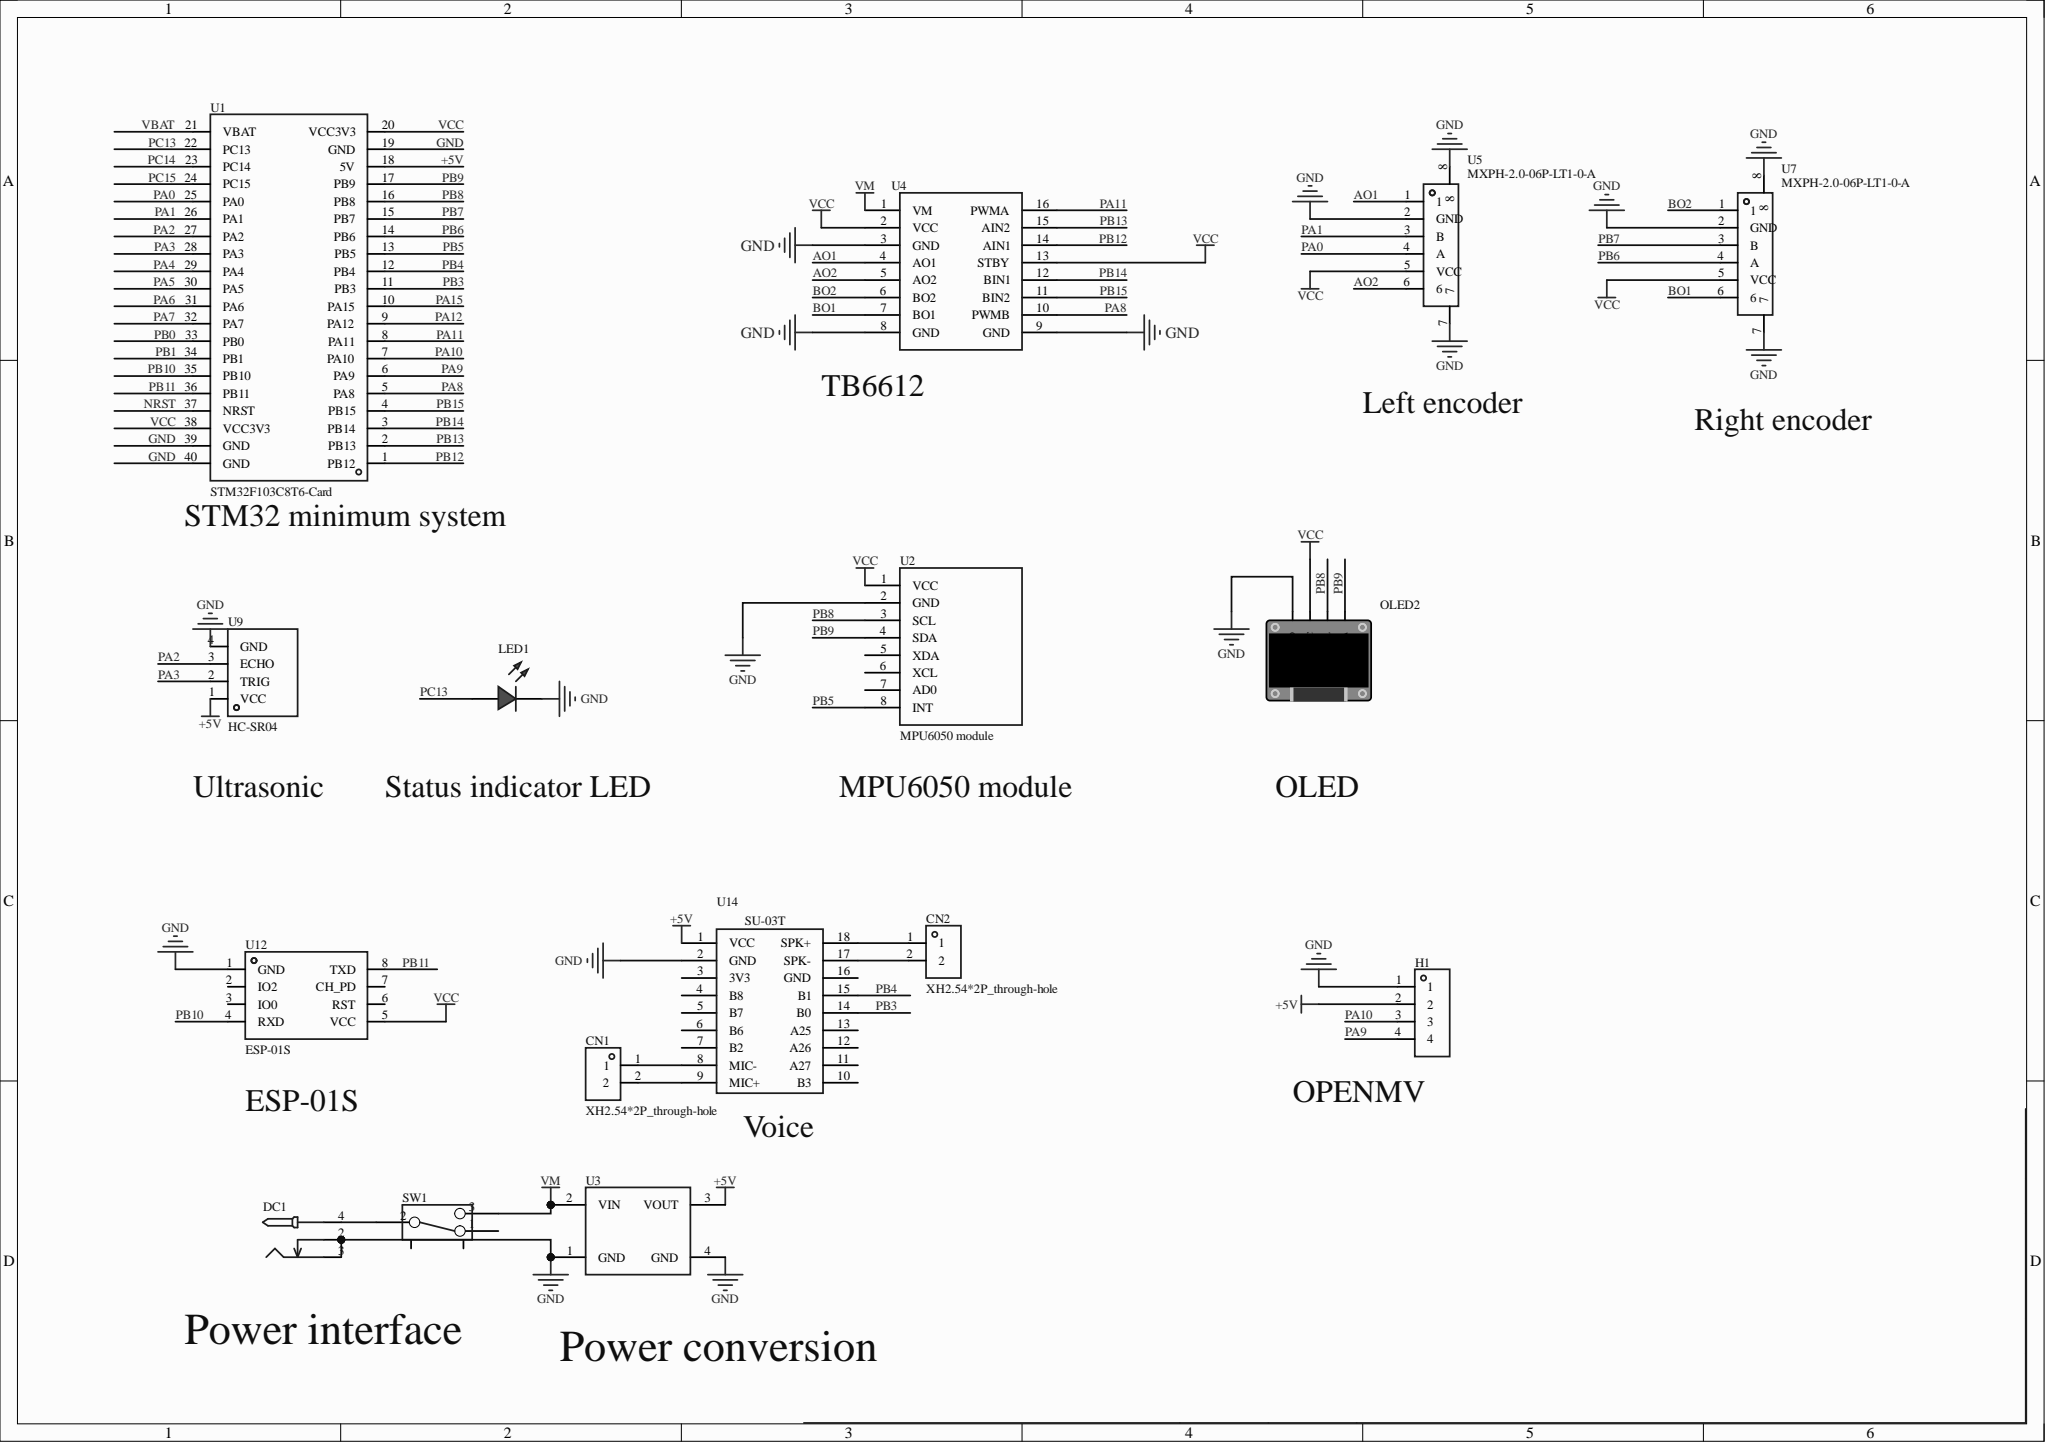Circuit board | Altium Designer | 16 parts | 35 nets
Bill of materials:
Comment,Description,Designator,Footprint,LibRef,Quantity
"XH2.54*2P_through-hole","","CN1, CN2","CONN-TH_2P-P2.50-XH2.54-2P","XH2.54*2P_直插","2"
"","","DC1","DC-2.0","DC-005_2.0","1"
"","","H1","HDR-TH_4P-P2.54-V-M","HDR-M_2.54_1x4P","1"
"","","LED1","LED_TH-3mm","LED_TH-R_3mm","1"
"","","OLED2","0.96OLED_4P","0.96OLED模块_4P","1"
"","","SW1","拨动开关","拨动开关_正","1"
"STM32F103C8T6-Card","","U1","CONN-TH_L53.3-W22.9_STM32F103C8T6-CARD","STM32F103C8T6-Card","1"
"MPU6050 module","","U2","MPU6050","MPU6050模块","1"
"","Adjustable output voltage, max 3A current","U3","MP1584主控","MP1584","1"
"","","U4","tb6612","tb6612","1"
"MXPH-2.0-06P-LT1-0-A","Pin structure:1x6P;pitch:2mm;mounting:vertical SMD;series:PH;total pins:6P;rows:1;pins per row:6;rated current:2A;contact material:copper alloy;contact plating:tin;operating temperature:-25℃~+85℃;","U5, U7","CONN-SMD_6P-P2.00_MXPH-2.0-6P-LT1-0-A","MXPH-2.0-06P-LT1-0-A","2"
"HC-SR04","","U9","TH_HC-SR04V","HC-SR04","1"
"ESP-01S","","U12","WIFIM-TH_ESP-01S","ESP-01S_C111009","1"
"","","U14","SU-03T","SU-03T","1"
Netlist (Protel format):
[
CN1
CONN-TH_2P-P2.50-XH2.54-2P
XH2.54*2P_through-hole



]
[
CN2
CONN-TH_2P-P2.50-XH2.54-2P
XH2.54*2P_through-hole



]
[
DC1
DC-2.0




]
[
H1
HDR-TH_4P-P2.54-V-M




]
[
LED1
LED_TH-3mm




]
[
OLED2
0.96OLED_4P




]
[
SW1
拨动开关




]
[
U1
CONN-TH_L53.3-W22.9_STM32F103C8T6-CARD
STM32F103C8T6-Card



]
[
U2
MPU6050
MPU6050 module



]
[
U3
MP1584主控




]
[
U4
tb6612




]
[
U5
CONN-SMD_6P-P2.00_MXPH-2.0-6P-LT1-0-A
MXPH-2.0-06P-LT1-0-A



]
[
U7
CONN-SMD_6P-P2.00_MXPH-2.0-6P-LT1-0-A
MXPH-2.0-06P-LT1-0-A



]
[
U9
TH_HC-SR04V
HC-SR04



]
[
U12
WIFIM-TH_ESP-01S
ESP-01S



]
[
U14
SU-03T




]
(
VM
SW1-3
U3-2
U4-1
)
(
VCC
OLED2-2
U1-20
U1-38
U2-1
U4-2
U4-13
U5-5
U7-5
U12-5
)
(
PC13
LED1-1
U1-22
)
(
PB15
U1-4
U4-11
)
(
PB14
U1-3
U4-12
)
(
PB13
U1-2
U4-15
)
(
PB12
U1-1
U4-14
)
(
PB11
U1-36
U12-8
)
(
PB10
U1-35
U12-4
)
(
PB9
OLED2-4
U1-17
U2-4
)
(
PB8
OLED2-3
U1-16
U2-3
)
(
PB7
U1-15
U7-3
)
(
PB6
U1-14
U7-4
)
(
PB5
U1-13
U2-8
)
(
PB4
U1-12
U14-15
)
(
PB3
U1-11
U14-14
)
(
PA11
U1-8
U4-16
)
(
PA10
H1-3
U1-7
)
(
PA9
H1-4
U1-6
)
(
PA8
U1-5
U4-10
)
(
PA3
U1-28
U9-2
)
(
PA2
U1-27
U9-3
)
(
PA1
U1-26
U5-3
)
(
PA0
U1-25
U5-4
)
(
NetDC1_4
DC1-4
SW1-2
)
(
NetCN2_2
CN2-2
U14-17
)
(
NetCN2_1
CN2-1
U14-18
)
(
NetCN1_2
CN1-2
U14-9
)
(
NetCN1_1
CN1-1
U14-8
)
(
GND
DC1-2
DC1-3
H1-1
LED1-2
OLED2-1
U1-19
U1-39
U1-40
U2-2
U3-1
U3-4
U4-3
U4-8
U4-9
U5-2
U5-7
U5-8
U7-2
U7-7
U7-8
U9-4
U12-1
U14-2
)
(
BO2
U4-6
U7-1
)
(
BO1
U4-7
U7-6
)
(
AO2
U4-5
U5-6
)
(
AO1
U4-4
U5-1
)
(
+5V
H1-2
U1-18
U3-3
U9-1
U14-1
)